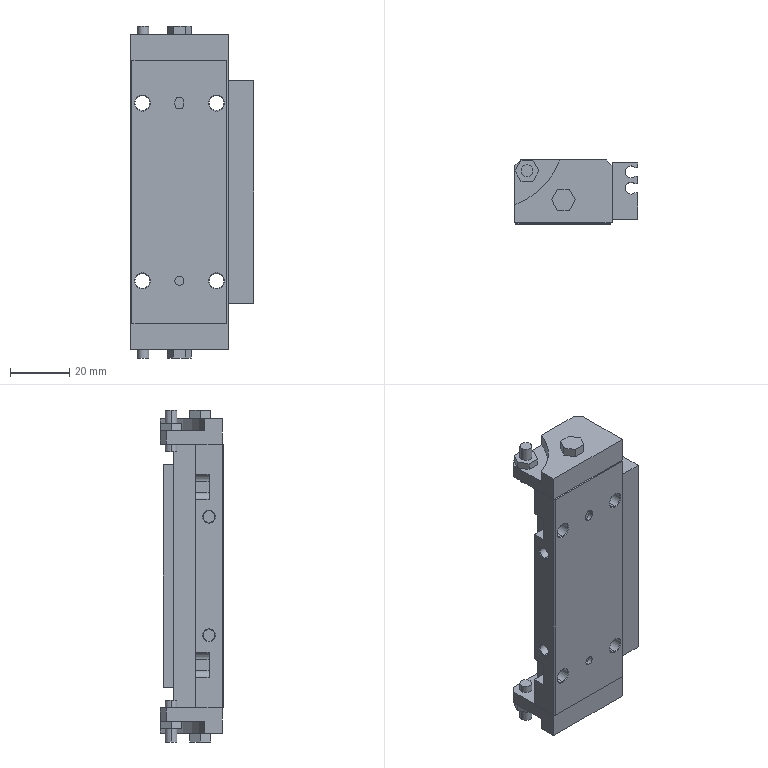Part | 1 solid | 177 faces | box 41.5 x 21.5 x 112 mm | volume 56399 mm3 | plane 102 | cylinder 47 | cone 28 | commonest cylinder face diameters 5 x20 4 x16 3 x9 50 x2